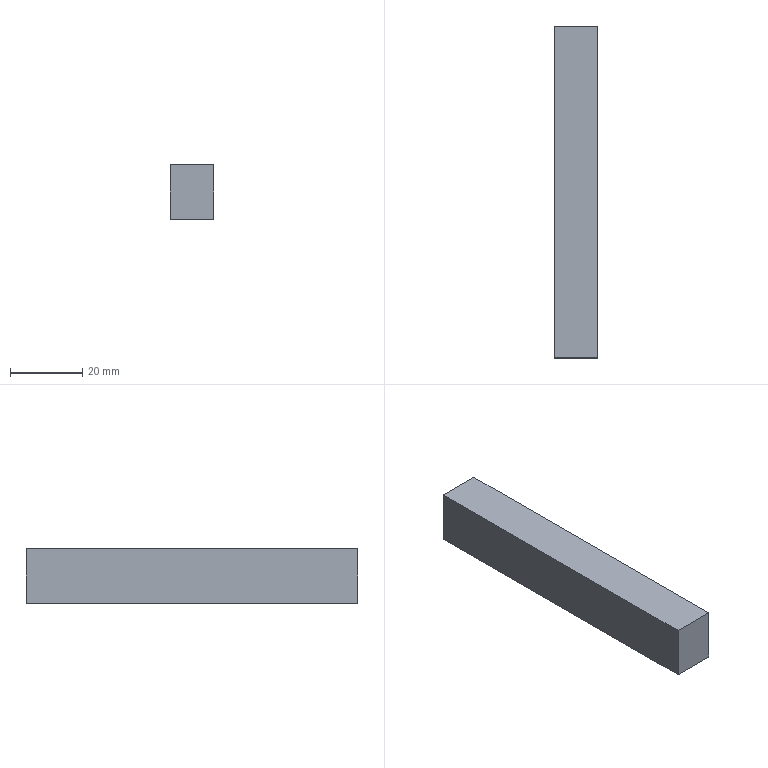Part | NX | features solid 2 | 1 solid | 6 faces | box 12 x 92 x 15 mm | volume 16560 mm3 | plane 6
STEP:
#1=CARTESIAN_POINT('',(-364.,-552.,-25.));
#2=VERTEX_POINT('',#1);
#3=CARTESIAN_POINT('',(-364.,-552.,-10.));
#4=VERTEX_POINT('',#3);
#5=CARTESIAN_POINT('',(-364.,-552.,64.523));
#6=DIRECTION('',(0.,0.,1.));
#7=VECTOR('',#6,1000.);
#8=LINE('',#5,#7);
#9=EDGE_CURVE('',#2,#4,#8,.T.);
#10=ORIENTED_EDGE('',*,*,#9,.T.);
#11=CARTESIAN_POINT('',(-352.,-552.,-10.));
#12=VERTEX_POINT('',#11);
#13=CARTESIAN_POINT('',(-203.,-552.,-10.));
#14=DIRECTION('',(1.,0.,0.));
#15=VECTOR('',#14,1000.);
#16=LINE('',#13,#15);
#17=EDGE_CURVE('',#4,#12,#16,.T.);
#18=ORIENTED_EDGE('',*,*,#17,.T.);
#19=CARTESIAN_POINT('',(-352.,-552.,-25.));
#20=VERTEX_POINT('',#19);
#21=CARTESIAN_POINT('',(-352.,-552.,64.523));
#22=DIRECTION('',(0.,0.,1.));
#23=VECTOR('',#22,1000.);
#24=LINE('',#21,#23);
#25=EDGE_CURVE('',#20,#12,#24,.T.);
#26=ORIENTED_EDGE('',*,*,#25,.F.);
#27=CARTESIAN_POINT('',(-385.,-552.,-25.));
#28=DIRECTION('',(-1.,0.,0.));
#29=VECTOR('',#28,1000.);
#30=LINE('',#27,#29);
#31=EDGE_CURVE('',#20,#2,#30,.T.);
#32=ORIENTED_EDGE('',*,*,#31,.T.);
#33=EDGE_LOOP('',(#10,#18,#26,#32));
#34=FACE_BOUND('',#33,.T.);
#35=CARTESIAN_POINT('',(-364.,-552.,-10.));
#36=DIRECTION('',(0.,1.,0.));
#37=DIRECTION('',(-1.,0.,0.));
#38=AXIS2_PLACEMENT_3D('',#35,#36,#37);
#39=PLANE('',#38);
#40=ADVANCED_FACE('',(#34),#39,.T.);
#41=CARTESIAN_POINT('',(-364.,-644.,-10.));
#42=VERTEX_POINT('',#41);
#43=CARTESIAN_POINT('',(-364.,-644.,-10.));
#44=DIRECTION('',(0.,1.,0.));
#45=VECTOR('',#44,1000.);
#46=LINE('',#43,#45);
#47=EDGE_CURVE('',#42,#4,#46,.T.);
#48=ORIENTED_EDGE('',*,*,#47,.F.);
#49=CARTESIAN_POINT('',(-352.,-644.,-10.));
#50=VERTEX_POINT('',#49);
#51=CARTESIAN_POINT('',(-385.,-644.,-10.));
#52=DIRECTION('',(1.,0.,0.));
#53=VECTOR('',#52,1000.);
#54=LINE('',#51,#53);
#55=EDGE_CURVE('',#42,#50,#54,.T.);
#56=ORIENTED_EDGE('',*,*,#55,.T.);
#57=CARTESIAN_POINT('',(-352.,-667.,-10.));
#58=DIRECTION('',(0.,-1.,0.));
#59=VECTOR('',#58,1000.);
#60=LINE('',#57,#59);
#61=EDGE_CURVE('',#12,#50,#60,.T.);
#62=ORIENTED_EDGE('',*,*,#61,.F.);
#63=ORIENTED_EDGE('',*,*,#17,.F.);
#64=EDGE_LOOP('',(#48,#56,#62,#63));
#65=FACE_BOUND('',#64,.T.);
#66=CARTESIAN_POINT('',(-385.,-577.,-10.));
#67=DIRECTION('',(0.,0.,1.));
#68=DIRECTION('',(1.,0.,0.));
#69=AXIS2_PLACEMENT_3D('',#66,#67,#68);
#70=PLANE('',#69);
#71=ADVANCED_FACE('',(#65),#70,.T.);
#72=ORIENTED_EDGE('',*,*,#9,.F.);
#73=CARTESIAN_POINT('',(-364.,-644.,-25.));
#74=VERTEX_POINT('',#73);
#75=CARTESIAN_POINT('',(-364.,-644.,-25.));
#76=DIRECTION('',(0.,-1.,0.));
#77=VECTOR('',#76,1000.);
#78=LINE('',#75,#77);
#79=EDGE_CURVE('',#2,#74,#78,.T.);
#80=ORIENTED_EDGE('',*,*,#79,.T.);
#81=CARTESIAN_POINT('',(-364.,-644.,64.523));
#82=DIRECTION('',(0.,0.,-1.));
#83=VECTOR('',#82,1000.);
#84=LINE('',#81,#83);
#85=EDGE_CURVE('',#42,#74,#84,.T.);
#86=ORIENTED_EDGE('',*,*,#85,.F.);
#87=ORIENTED_EDGE('',*,*,#47,.T.);
#88=EDGE_LOOP('',(#72,#80,#86,#87));
#89=FACE_BOUND('',#88,.T.);
#90=CARTESIAN_POINT('',(-364.,-644.,64.523));
#91=DIRECTION('',(1.,0.,0.));
#92=DIRECTION('',(0.,1.,0.));
#93=AXIS2_PLACEMENT_3D('',#90,#91,#92);
#94=PLANE('',#93);
#95=ADVANCED_FACE('',(#89),#94,.F.);
#96=CARTESIAN_POINT('',(-352.,-644.,-25.));
#97=VERTEX_POINT('',#96);
#98=CARTESIAN_POINT('',(-352.,-644.,-25.));
#99=DIRECTION('',(0.,-1.,0.));
#100=VECTOR('',#99,1000.);
#101=LINE('',#98,#100);
#102=EDGE_CURVE('',#20,#97,#101,.T.);
#103=ORIENTED_EDGE('',*,*,#102,.F.);
#104=ORIENTED_EDGE('',*,*,#25,.T.);
#105=ORIENTED_EDGE('',*,*,#61,.T.);
#106=CARTESIAN_POINT('',(-352.,-644.,64.523));
#107=DIRECTION('',(0.,0.,-1.));
#108=VECTOR('',#107,1000.);
#109=LINE('',#106,#108);
#110=EDGE_CURVE('',#50,#97,#109,.T.);
#111=ORIENTED_EDGE('',*,*,#110,.T.);
#112=EDGE_LOOP('',(#103,#104,#105,#111));
#113=FACE_BOUND('',#112,.T.);
#114=CARTESIAN_POINT('',(-352.,-644.,64.523));
#115=DIRECTION('',(1.,0.,0.));
#116=DIRECTION('',(0.,1.,0.));
#117=AXIS2_PLACEMENT_3D('',#114,#115,#116);
#118=PLANE('',#117);
#119=ADVANCED_FACE('',(#113),#118,.T.);
#120=CARTESIAN_POINT('',(-385.,-644.,-25.));
#121=DIRECTION('',(1.,0.,0.));
#122=VECTOR('',#121,1000.);
#123=LINE('',#120,#122);
#124=EDGE_CURVE('',#74,#97,#123,.T.);
#125=ORIENTED_EDGE('',*,*,#124,.F.);
#126=ORIENTED_EDGE('',*,*,#79,.F.);
#127=ORIENTED_EDGE('',*,*,#31,.F.);
#128=ORIENTED_EDGE('',*,*,#102,.T.);
#129=EDGE_LOOP('',(#125,#126,#127,#128));
#130=FACE_BOUND('',#129,.T.);
#131=CARTESIAN_POINT('',(-385.,-577.,-25.));
#132=DIRECTION('',(0.,0.,1.));
#133=DIRECTION('',(1.,0.,0.));
#134=AXIS2_PLACEMENT_3D('',#131,#132,#133);
#135=PLANE('',#134);
#136=ADVANCED_FACE('',(#130),#135,.F.);
#137=ORIENTED_EDGE('',*,*,#55,.F.);
#138=ORIENTED_EDGE('',*,*,#85,.T.);
#139=ORIENTED_EDGE('',*,*,#124,.T.);
#140=ORIENTED_EDGE('',*,*,#110,.F.);
#141=EDGE_LOOP('',(#137,#138,#139,#140));
#142=FACE_BOUND('',#141,.T.);
#143=CARTESIAN_POINT('',(-364.,-644.,-10.));
#144=DIRECTION('',(0.,-1.,0.));
#145=DIRECTION('',(0.,0.,-1.));
#146=AXIS2_PLACEMENT_3D('',#143,#144,#145);
#147=PLANE('',#146);
#148=ADVANCED_FACE('',(#142),#147,.T.);
#149=CLOSED_SHELL('',(#40,#71,#95,#119,#136,#148));
#150=MANIFOLD_SOLID_BREP('',#149);
#151=(LENGTH_UNIT()NAMED_UNIT(*)SI_UNIT(.MILLI.,.METRE.));
#152=UNCERTAINTY_MEASURE_WITH_UNIT(LENGTH_MEASURE(0.00001),#151,'','');
#153=(NAMED_UNIT(*)PLANE_ANGLE_UNIT()SI_UNIT($,.RADIAN.));
#154=(NAMED_UNIT(*)SI_UNIT($,.STERADIAN.)SOLID_ANGLE_UNIT());
#155=(GEOMETRIC_REPRESENTATION_CONTEXT(3)GLOBAL_UNCERTAINTY_ASSIGNED_CONTEXT((#152))GLOBAL_UNIT_ASSIGNED_CONTEXT((#151,#153,#154))REPRESENTATION_CONTEXT('',''));
#156=ADVANCED_BREP_SHAPE_REPRESENTATION('',(#150),#155);